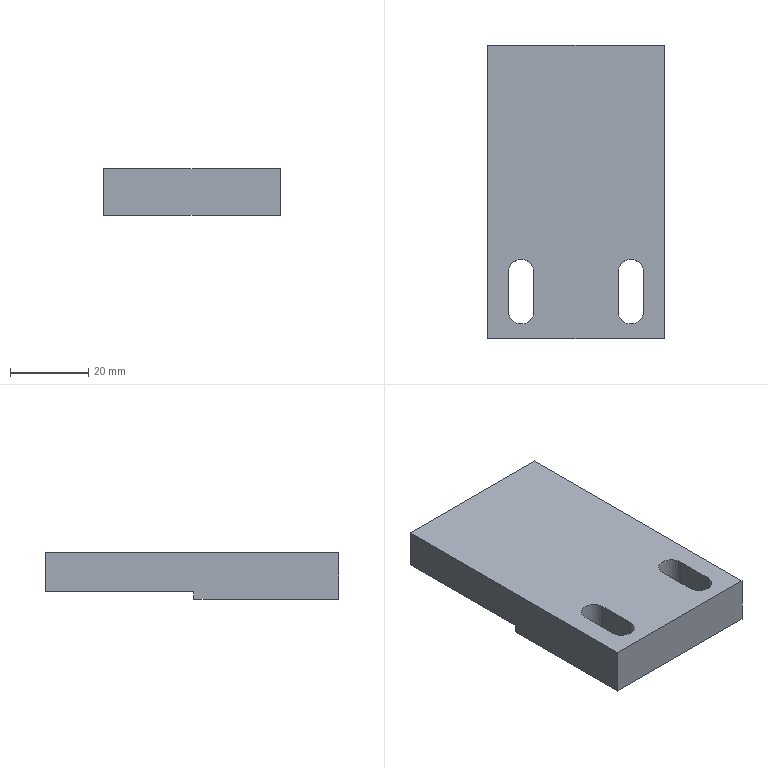Part | STEP file | detection cylinder seat support plate--1 | 1 solid | 24 faces | box 45 x 75 x 12 mm | volume 34324 mm3 | plane 12 | cylinder 8 | cone 4 | commonest cylinder face diameters 4.2 x4 6.5 x4